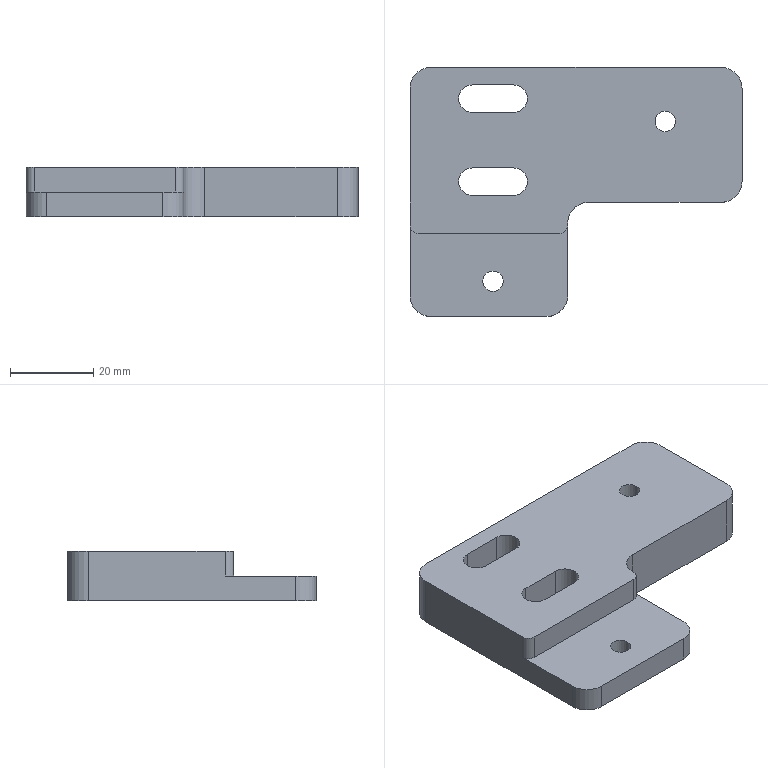NC program | NX | posted with a generic post | part box 80 x 60 x 12 mm
Whole program:
N10 G17 G21 G94 G90
(FLOOR_WALL_COPY , TOOL : D80)
N12 T19 M6
N14 G54
N16 G17 G0 G90 X-85. Y0. S6500 M3
N18 G43 Z30. H19
N20 Z5.
N22 G94 G1 Z2. F1500.
N24 X-82.
N26 X82.
N28 X85.
N30 Z5.
N32 G0 Z30.
N34 X-85.
N36 Z4.
N38 G1 Z1.
N40 X-82.
N42 X82.
N44 X85.
N46 Z4.
N48 G0 Z30.
N50 X-85.
N52 Z3.
N54 G1 Z0.
N56 X-82.
N58 X82.
N60 X85.
N62 Z3.
N64 G0 Z30.
N66 M5
(PLANAR_MILL_COPY_COPY_COPY_COPY_1 , TOOL : D6A45)
N68 T01 M6
N70 G54
N72 G17 G0 G90 X19.134 Y-22.559 S9500 M3
N74 G43 Z30. H1
N76 Z0.5
N78 G94 G1 Z-1. F1250.
N80 G3 X20. Y-23.059 R1.
N82 X21.559 Y-21.5 R1.559
N84 X20. Y-23.059 R-1.559
N86 X20.866 Y-22.559 R1.
N88 G1 Z0.5
N90 G0 Z30.
N92 X19.134 Y0.6
N94 Z0.5
N96 G1 Z-1.
N98 G3 X20. Y0.1 R1.
N100 G1 X25.
N102 G3 X27.4 Y2.5 R2.4
N104 X25. Y4.9 R2.4
N106 G1 X15.
N108 G3 X12.6 Y2.5 R2.4
N110 X15. Y0.1 R2.4
N112 G1 X20.
N114 G3 X20.866 Y0.6 R1.
N116 G1 Z0.5
N118 G0 Z30.
N120 Y24.4
N122 Z0.5
N124 G1 Z-1.
N126 G3 X20. Y24.9 R1.
N128 G1 X15.
N130 G3 X12.6 Y22.5 R2.4
N132 X15. Y20.1 R2.4
N134 G1 X25.
N136 G3 X27.4 Y22.5 R2.4
N138 X25. Y24.9 R2.4
N140 G1 X20.
N142 G3 X19.134 Y24.4 R1.
N144 G1 Z0.5
N146 G0 Z30.
N148 X-0.866 Y31.4
N150 Z0.5
N152 G1 Z-1.
N154 G3 X0. Y30.9 R1.
N156 G1 X35.
N158 G2 X40.9 Y25. R5.9
N160 G1 Y-25.
N162 G2 X35. Y-30.9 R5.9
N164 G1 X7.
N166 G2 X1.1 Y-25. R5.9
N168 G1 Y-7.5
N170 G3 X-3. Y-3.4 R4.1
N172 G1 X-35.
N174 G2 X-40.9 Y2.5 R5.9
N176 G1 Y25.
N178 G2 X-35. Y30.9 R5.9
N180 G1 X0.
N182 G3 X0.866 Y31.4 R1.
N184 G1 Z0.5
N186 G0 Z30.
N188 X-20.634 Y18.059
N190 Z0.5
N192 G1 Z-1.
N194 G3 X-21.5 Y18.559 R1.
N196 X-23.059 Y17. R1.559
N198 X-21.5 Y18.559 R-1.559
N200 X-22.366 Y18.059 R1.
N202 G1 Z0.5
N204 G0 Z30.
N206 M5
N208 M2